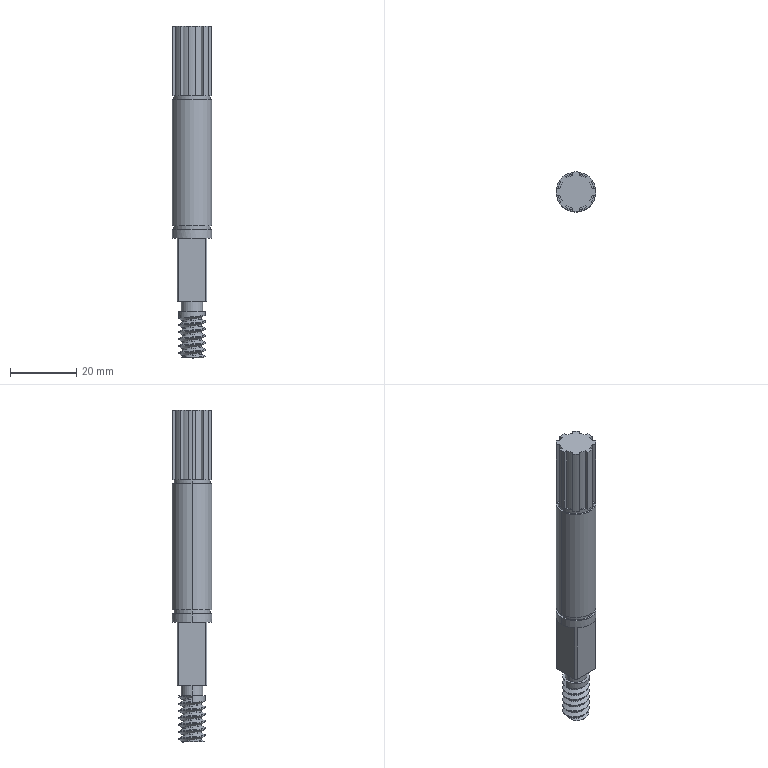Part | SolidWorks | features ICE 7, Chamfer 1, Extrusion 1, SweepThread 1 | 1 solid | 94 faces | box 12 x 12 x 100 mm | volume 8949 mm3 | plane 48 | cylinder 41 | spline 3 | cone 2 | commonest cylinder face diameters 8 x14 12 x13 10 x8 11 x4 6.5 x2